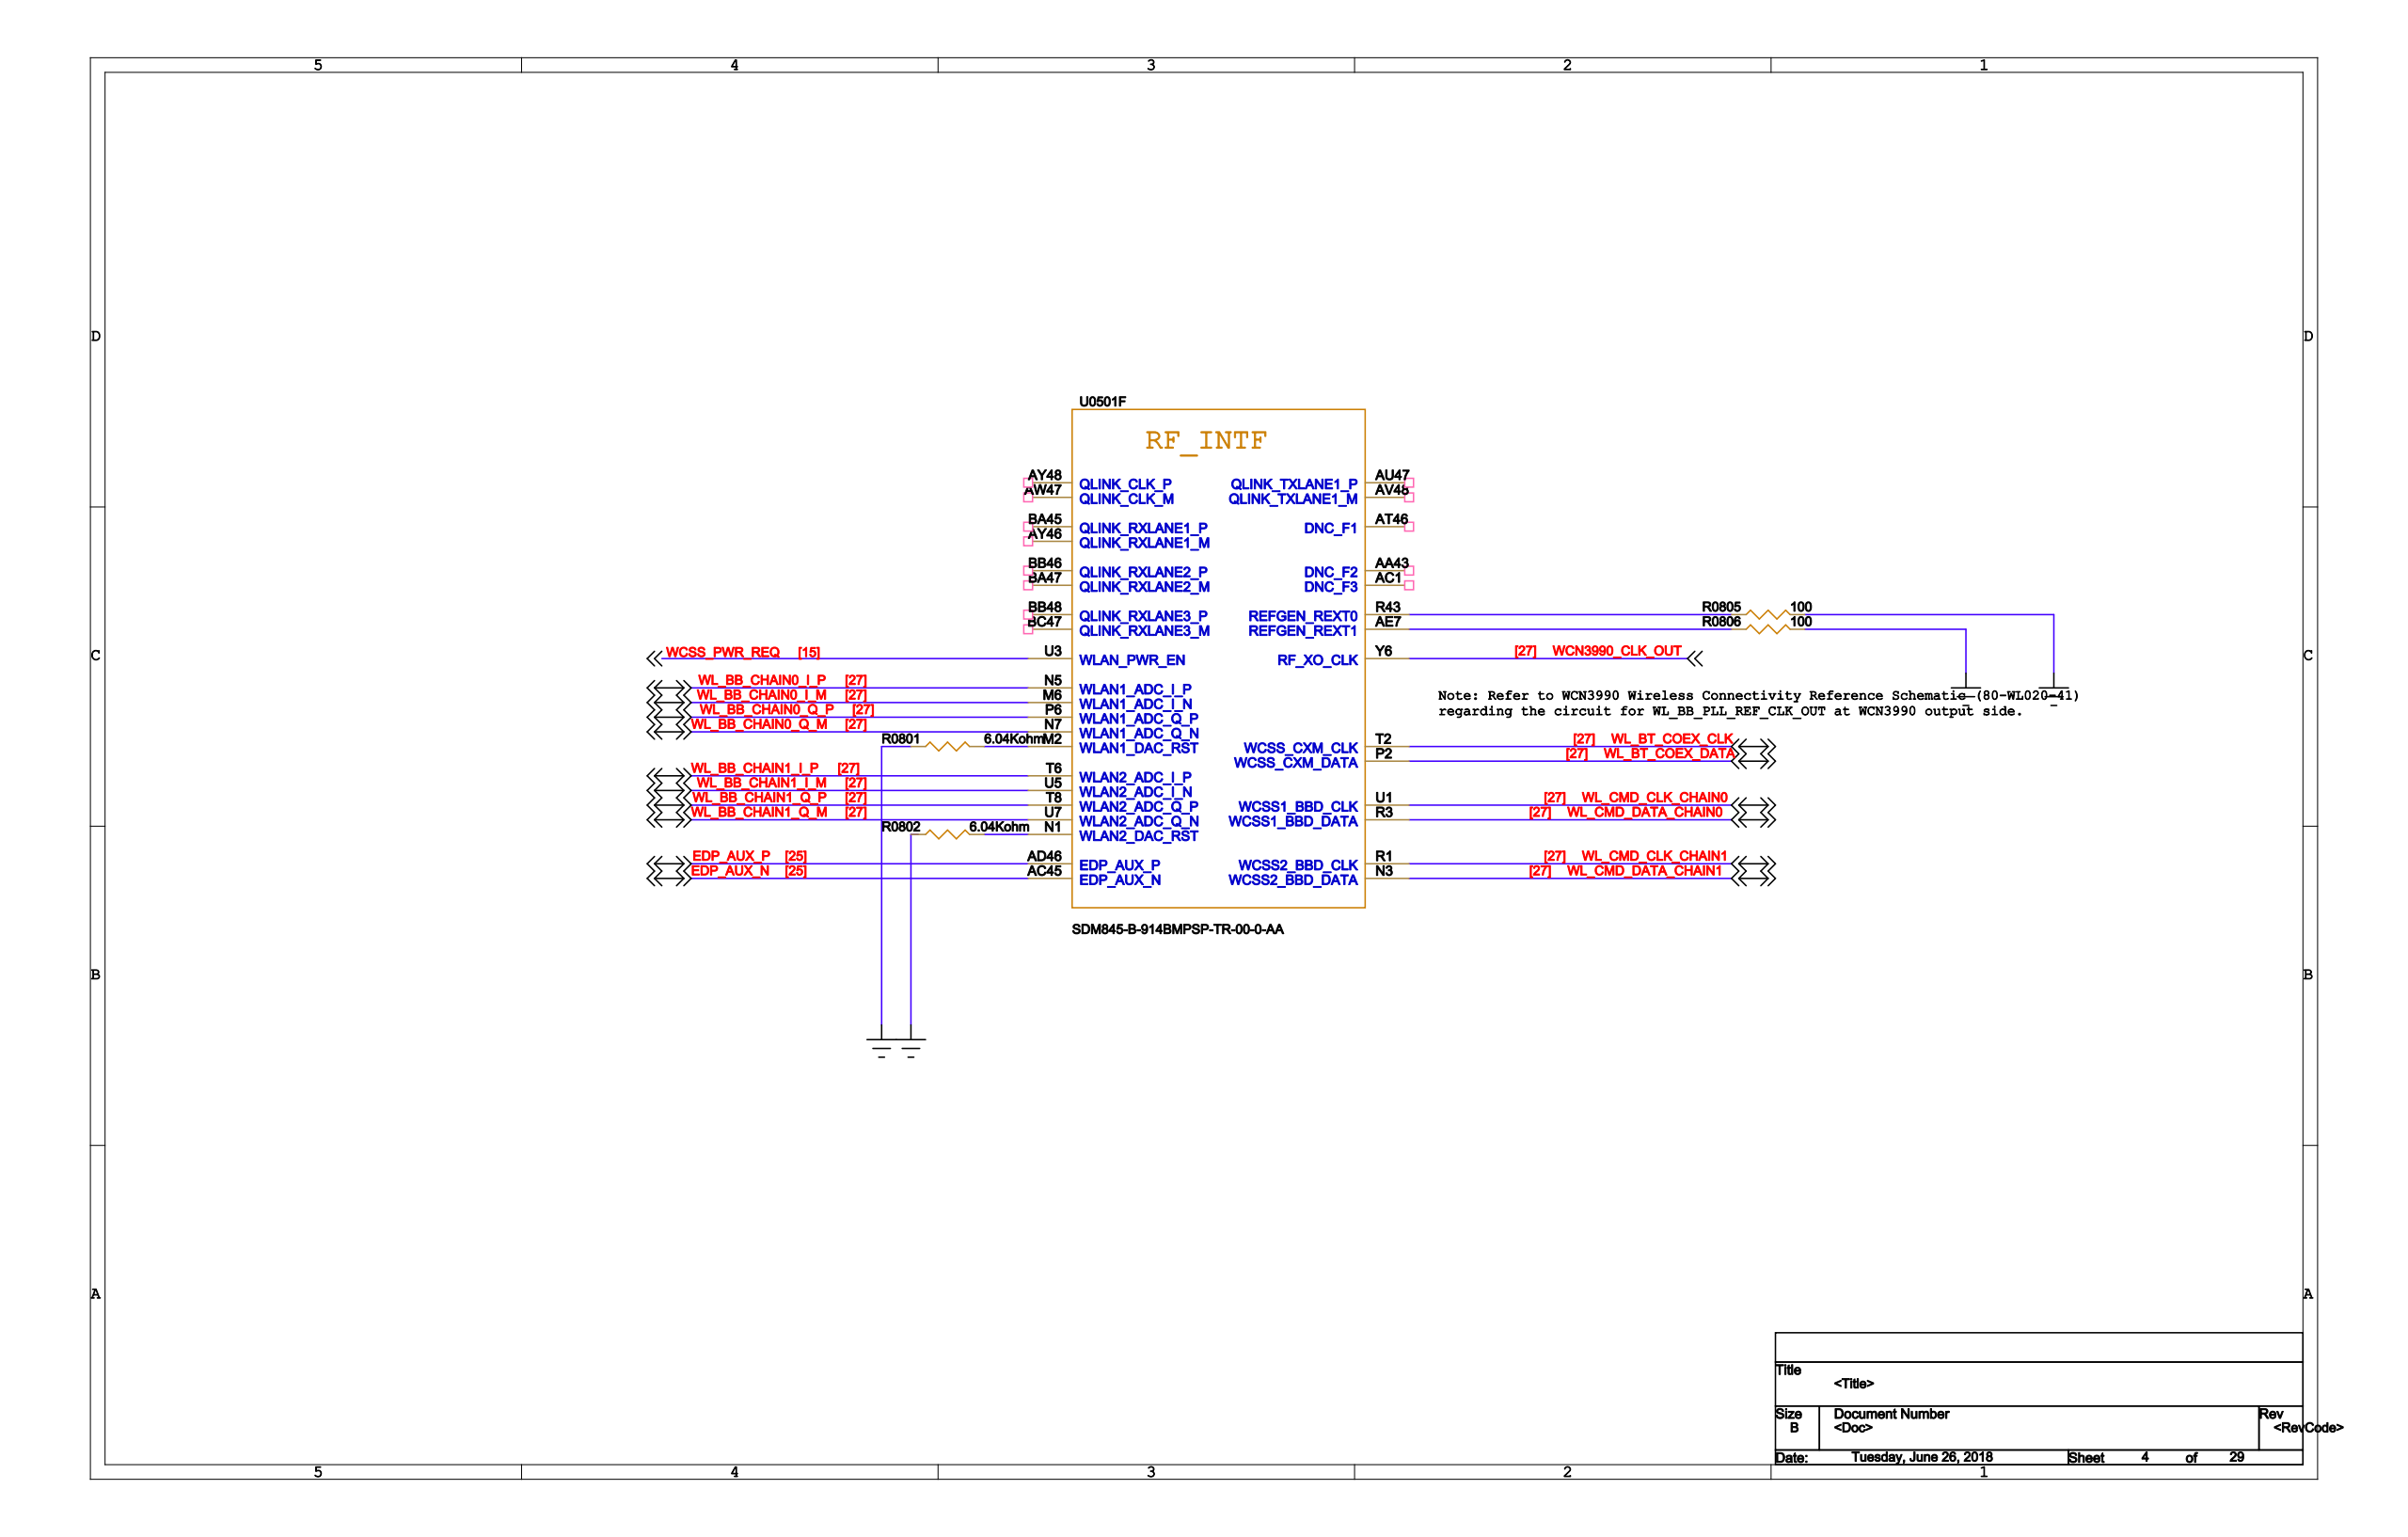Circuit board | Cadence Allegro | 802 parts | 566 nets | one sheet of the schematic
Parts on this sheet (reference | value | footprint):
R0801 | 6.04Kohm | R0201
R0802 | 6.04Kohm | R0201
R0805 | 100 | R0201
R0806 | 100 | R0201
U0501 | SDM845-B-914BMPSP-TR-00-0-AA | BGA914_12P4X12P4_0P58_0P35
Nets of these parts (net: part-pin ...):
GND: R0801-1 R0802-1 R0805-2 R0806-2
EDP_AUX_P: U0501-AD46
EDP_AUX_N: U0501-AC45
WL_CMD_CLK_CHAIN0: U0501-U1
WL_CMD_DATA_CHAIN0: U0501-R3
WL_CMD_CLK_CHAIN1: U0501-R1
WL_CMD_DATA_CHAIN1: U0501-N3
N57153: R0801-2 U0501-M2
N56583: R0802-2 U0501-N1
N56192: R0805-1 U0501-R43
N56196: R0806-1 U0501-AE7
WCN3990_CLK_OUT: U0501-Y6
WL_BT_COEX_CLK: U0501-T2
WL_BT_COEX_DATA: U0501-P2
WL_BB_CHAIN0_I_M: U0501-M6
WL_BB_CHAIN0_I_P: U0501-N5
WL_BB_CHAIN0_Q_M: U0501-N7
WL_BB_CHAIN0_Q_P: U0501-P6
WL_BB_CHAIN1_I_M: U0501-U5
WL_BB_CHAIN1_I_P: U0501-T6
WL_BB_CHAIN1_Q_M: U0501-U7
WL_BB_CHAIN1_Q_P: U0501-T8
WCSS_PWR_REQ: U0501-U3